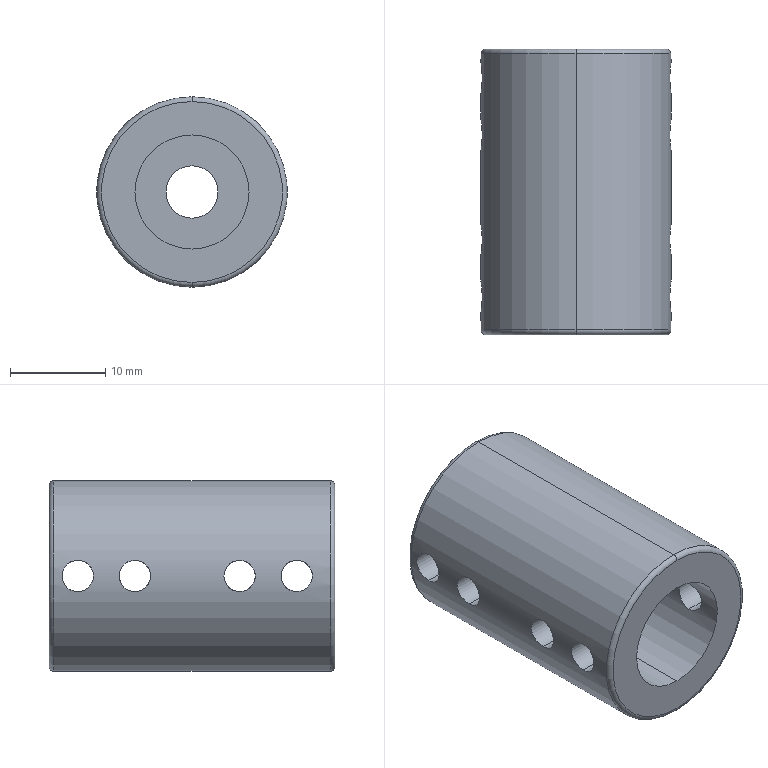Part | SolidWorks | features ICE 2, 3DProfileFeature 1, Extrusion 1, Fillet 1, HoleWzd 1 | 1 solid | 29 faces | box 20 x 30 x 20 mm | volume 6976 mm3 | cylinder 22 | torus 4 | plane 3 | commonest cylinder face diameters 3.3 x16 5.5 x2 12 x2 20 x2